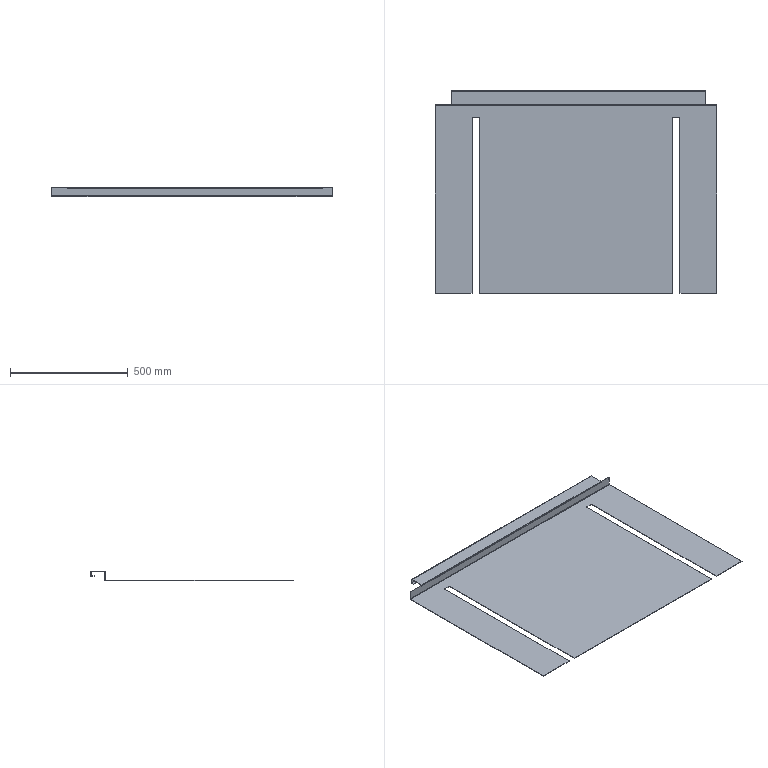Part | SolidWorks | features BaseBody 1 | 1 solid | 54 faces | box 1196 x 863 x 39 mm | volume 2108155 mm3 | plane 46 | cylinder 8 | commonest cylinder face diameters 2 x4 6 x4
STEP:
#1=CARTESIAN_POINT('',(412.5,349.,-2.));
#2=VERTEX_POINT('',#1);
#3=CARTESIAN_POINT('',(442.5,349.,-2.));
#4=VERTEX_POINT('',#3);
#5=CARTESIAN_POINT('',(412.5,349.,-2.));
#6=DIRECTION('',(1.,0.,0.));
#7=VECTOR('',#6,1000.);
#8=LINE('',#5,#7);
#9=EDGE_CURVE('',#2,#4,#8,.T.);
#10=ORIENTED_EDGE('',*,*,#9,.T.);
#11=CARTESIAN_POINT('',(442.5,349.,0.));
#12=VERTEX_POINT('',#11);
#13=CARTESIAN_POINT('',(442.5,349.,0.));
#14=DIRECTION('',(0.,0.,-1.));
#15=VECTOR('',#14,1000.);
#16=LINE('',#13,#15);
#17=EDGE_CURVE('',#12,#4,#16,.T.);
#18=ORIENTED_EDGE('',*,*,#17,.F.);
#19=CARTESIAN_POINT('',(412.5,349.,0.));
#20=VERTEX_POINT('',#19);
#21=CARTESIAN_POINT('',(412.5,349.,0.));
#22=DIRECTION('',(1.,0.,0.));
#23=VECTOR('',#22,1000.);
#24=LINE('',#21,#23);
#25=EDGE_CURVE('',#20,#12,#24,.T.);
#26=ORIENTED_EDGE('',*,*,#25,.F.);
#27=CARTESIAN_POINT('',(412.5,349.,0.));
#28=DIRECTION('',(0.,0.,-1.));
#29=VECTOR('',#28,1000.);
#30=LINE('',#27,#29);
#31=EDGE_CURVE('',#20,#2,#30,.T.);
#32=ORIENTED_EDGE('',*,*,#31,.T.);
#33=EDGE_LOOP('',(#10,#18,#26,#32));
#34=FACE_OUTER_BOUND('',#33,.T.);
#35=CARTESIAN_POINT('',(412.5,349.,0.));
#36=DIRECTION('',(0.,1.,0.));
#37=DIRECTION('',(1.,0.,0.));
#38=AXIS2_PLACEMENT_3D('',#35,#36,#37);
#39=PLANE('',#38);
#40=ADVANCED_FACE('',(#34),#39,.F.);
#41=CARTESIAN_POINT('',(442.5,-401.,-2.));
#42=VERTEX_POINT('',#41);
#43=CARTESIAN_POINT('',(442.5,349.,-2.));
#44=DIRECTION('',(0.,-1.,0.));
#45=VECTOR('',#44,1000.);
#46=LINE('',#43,#45);
#47=EDGE_CURVE('',#4,#42,#46,.T.);
#48=ORIENTED_EDGE('',*,*,#47,.T.);
#49=CARTESIAN_POINT('',(442.5,-401.,0.));
#50=VERTEX_POINT('',#49);
#51=CARTESIAN_POINT('',(442.5,-401.,0.));
#52=DIRECTION('',(0.,0.,-1.));
#53=VECTOR('',#52,1000.);
#54=LINE('',#51,#53);
#55=EDGE_CURVE('',#50,#42,#54,.T.);
#56=ORIENTED_EDGE('',*,*,#55,.F.);
#57=CARTESIAN_POINT('',(442.5,349.,0.));
#58=DIRECTION('',(0.,-1.,0.));
#59=VECTOR('',#58,1000.);
#60=LINE('',#57,#59);
#61=EDGE_CURVE('',#12,#50,#60,.T.);
#62=ORIENTED_EDGE('',*,*,#61,.F.);
#63=ORIENTED_EDGE('',*,*,#17,.T.);
#64=EDGE_LOOP('',(#48,#56,#62,#63));
#65=FACE_OUTER_BOUND('',#64,.T.);
#66=CARTESIAN_POINT('',(442.5,349.,0.));
#67=DIRECTION('',(1.,0.,0.));
#68=DIRECTION('',(0.,-1.,0.));
#69=AXIS2_PLACEMENT_3D('',#66,#67,#68);
#70=PLANE('',#69);
#71=ADVANCED_FACE('',(#65),#70,.F.);
#72=CARTESIAN_POINT('',(412.5,-401.,-2.));
#73=VERTEX_POINT('',#72);
#74=CARTESIAN_POINT('',(412.5,349.,-2.));
#75=DIRECTION('',(0.,1.,0.));
#76=VECTOR('',#75,1000.);
#77=LINE('',#74,#76);
#78=EDGE_CURVE('',#73,#2,#77,.T.);
#79=ORIENTED_EDGE('',*,*,#78,.T.);
#80=ORIENTED_EDGE('',*,*,#31,.F.);
#81=CARTESIAN_POINT('',(412.5,-401.,0.));
#82=VERTEX_POINT('',#81);
#83=CARTESIAN_POINT('',(412.5,349.,0.));
#84=DIRECTION('',(0.,1.,0.));
#85=VECTOR('',#84,1000.);
#86=LINE('',#83,#85);
#87=EDGE_CURVE('',#82,#20,#86,.T.);
#88=ORIENTED_EDGE('',*,*,#87,.F.);
#89=CARTESIAN_POINT('',(412.5,-401.,0.));
#90=DIRECTION('',(0.,0.,-1.));
#91=VECTOR('',#90,1000.);
#92=LINE('',#89,#91);
#93=EDGE_CURVE('',#82,#73,#92,.T.);
#94=ORIENTED_EDGE('',*,*,#93,.T.);
#95=EDGE_LOOP('',(#79,#80,#88,#94));
#96=FACE_OUTER_BOUND('',#95,.T.);
#97=CARTESIAN_POINT('',(412.5,349.,0.));
#98=DIRECTION('',(-1.,0.,0.));
#99=DIRECTION('',(0.,0.,1.));
#100=AXIS2_PLACEMENT_3D('',#97,#98,#99);
#101=PLANE('',#100);
#102=ADVANCED_FACE('',(#96),#101,.F.);
#103=CARTESIAN_POINT('',(-442.5,349.,-2.));
#104=VERTEX_POINT('',#103);
#105=CARTESIAN_POINT('',(-412.5,349.,-2.));
#106=VERTEX_POINT('',#105);
#107=CARTESIAN_POINT('',(-412.5,349.,-2.));
#108=DIRECTION('',(1.,0.,0.));
#109=VECTOR('',#108,1000.);
#110=LINE('',#107,#109);
#111=EDGE_CURVE('',#104,#106,#110,.T.);
#112=ORIENTED_EDGE('',*,*,#111,.T.);
#113=CARTESIAN_POINT('',(-412.5,349.,0.));
#114=VERTEX_POINT('',#113);
#115=CARTESIAN_POINT('',(-412.5,349.,0.));
#116=DIRECTION('',(0.,0.,-1.));
#117=VECTOR('',#116,1000.);
#118=LINE('',#115,#117);
#119=EDGE_CURVE('',#114,#106,#118,.T.);
#120=ORIENTED_EDGE('',*,*,#119,.F.);
#121=CARTESIAN_POINT('',(-442.5,349.,0.));
#122=VERTEX_POINT('',#121);
#123=CARTESIAN_POINT('',(-412.5,349.,0.));
#124=DIRECTION('',(1.,0.,0.));
#125=VECTOR('',#124,1000.);
#126=LINE('',#123,#125);
#127=EDGE_CURVE('',#122,#114,#126,.T.);
#128=ORIENTED_EDGE('',*,*,#127,.F.);
#129=CARTESIAN_POINT('',(-442.5,349.,0.));
#130=DIRECTION('',(0.,0.,-1.));
#131=VECTOR('',#130,1000.);
#132=LINE('',#129,#131);
#133=EDGE_CURVE('',#122,#104,#132,.T.);
#134=ORIENTED_EDGE('',*,*,#133,.T.);
#135=EDGE_LOOP('',(#112,#120,#128,#134));
#136=FACE_OUTER_BOUND('',#135,.T.);
#137=CARTESIAN_POINT('',(-412.5,349.,0.));
#138=DIRECTION('',(0.,1.,0.));
#139=DIRECTION('',(1.,0.,0.));
#140=AXIS2_PLACEMENT_3D('',#137,#138,#139);
#141=PLANE('',#140);
#142=ADVANCED_FACE('',(#136),#141,.F.);
#143=CARTESIAN_POINT('',(-412.5,-401.,-2.));
#144=VERTEX_POINT('',#143);
#145=CARTESIAN_POINT('',(-412.5,349.,-2.));
#146=DIRECTION('',(0.,-1.,0.));
#147=VECTOR('',#146,1000.);
#148=LINE('',#145,#147);
#149=EDGE_CURVE('',#106,#144,#148,.T.);
#150=ORIENTED_EDGE('',*,*,#149,.T.);
#151=CARTESIAN_POINT('',(-412.5,-401.,0.));
#152=VERTEX_POINT('',#151);
#153=CARTESIAN_POINT('',(-412.5,-401.,0.));
#154=DIRECTION('',(0.,0.,-1.));
#155=VECTOR('',#154,1000.);
#156=LINE('',#153,#155);
#157=EDGE_CURVE('',#152,#144,#156,.T.);
#158=ORIENTED_EDGE('',*,*,#157,.F.);
#159=CARTESIAN_POINT('',(-412.5,349.,0.));
#160=DIRECTION('',(0.,-1.,0.));
#161=VECTOR('',#160,1000.);
#162=LINE('',#159,#161);
#163=EDGE_CURVE('',#114,#152,#162,.T.);
#164=ORIENTED_EDGE('',*,*,#163,.F.);
#165=ORIENTED_EDGE('',*,*,#119,.T.);
#166=EDGE_LOOP('',(#150,#158,#164,#165));
#167=FACE_OUTER_BOUND('',#166,.T.);
#168=CARTESIAN_POINT('',(-412.5,349.,0.));
#169=DIRECTION('',(1.,0.,0.));
#170=DIRECTION('',(0.,-1.,0.));
#171=AXIS2_PLACEMENT_3D('',#168,#169,#170);
#172=PLANE('',#171);
#173=ADVANCED_FACE('',(#167),#172,.F.);
#174=CARTESIAN_POINT('',(-442.5,-401.,-2.));
#175=VERTEX_POINT('',#174);
#176=CARTESIAN_POINT('',(-442.5,349.,-2.));
#177=DIRECTION('',(0.,1.,0.));
#178=VECTOR('',#177,1000.);
#179=LINE('',#176,#178);
#180=EDGE_CURVE('',#175,#104,#179,.T.);
#181=ORIENTED_EDGE('',*,*,#180,.T.);
#182=ORIENTED_EDGE('',*,*,#133,.F.);
#183=CARTESIAN_POINT('',(-442.5,-401.,0.));
#184=VERTEX_POINT('',#183);
#185=CARTESIAN_POINT('',(-442.5,349.,0.));
#186=DIRECTION('',(0.,1.,0.));
#187=VECTOR('',#186,1000.);
#188=LINE('',#185,#187);
#189=EDGE_CURVE('',#184,#122,#188,.T.);
#190=ORIENTED_EDGE('',*,*,#189,.F.);
#191=CARTESIAN_POINT('',(-442.5,-401.,0.));
#192=DIRECTION('',(0.,0.,-1.));
#193=VECTOR('',#192,1000.);
#194=LINE('',#191,#193);
#195=EDGE_CURVE('',#184,#175,#194,.T.);
#196=ORIENTED_EDGE('',*,*,#195,.T.);
#197=EDGE_LOOP('',(#181,#182,#190,#196));
#198=FACE_OUTER_BOUND('',#197,.T.);
#199=CARTESIAN_POINT('',(-442.5,349.,0.));
#200=DIRECTION('',(-1.,0.,0.));
#201=DIRECTION('',(0.,0.,1.));
#202=AXIS2_PLACEMENT_3D('',#199,#200,#201);
#203=PLANE('',#202);
#204=ADVANCED_FACE('',(#198),#203,.F.);
#205=CARTESIAN_POINT('',(-528.,447.,19.));
#206=VERTEX_POINT('',#205);
#207=CARTESIAN_POINT('',(553.,447.,19.));
#208=VERTEX_POINT('',#207);
#209=CARTESIAN_POINT('',(0.,447.,19.));
#210=DIRECTION('',(1.,0.,0.));
#211=VECTOR('',#210,1000.);
#212=LINE('',#209,#211);
#213=EDGE_CURVE('',#206,#208,#212,.T.);
#214=ORIENTED_EDGE('',*,*,#213,.F.);
#215=CARTESIAN_POINT('',(-528.,447.,17.));
#216=VERTEX_POINT('',#215);
#217=CARTESIAN_POINT('',(-528.,447.,17.));
#218=DIRECTION('',(0.,0.,1.));
#219=VECTOR('',#218,1000.);
#220=LINE('',#217,#219);
#221=EDGE_CURVE('',#216,#206,#220,.T.);
#222=ORIENTED_EDGE('',*,*,#221,.F.);
#223=CARTESIAN_POINT('',(553.,447.,17.));
#224=VERTEX_POINT('',#223);
#225=CARTESIAN_POINT('',(553.,447.,17.));
#226=DIRECTION('',(1.,0.,0.));
#227=VECTOR('',#226,1000.);
#228=LINE('',#225,#227);
#229=EDGE_CURVE('',#216,#224,#228,.T.);
#230=ORIENTED_EDGE('',*,*,#229,.T.);
#231=CARTESIAN_POINT('',(553.,447.,17.));
#232=DIRECTION('',(0.,0.,1.));
#233=VECTOR('',#232,1000.);
#234=LINE('',#231,#233);
#235=EDGE_CURVE('',#224,#208,#234,.T.);
#236=ORIENTED_EDGE('',*,*,#235,.T.);
#237=EDGE_LOOP('',(#214,#222,#230,#236));
#238=FACE_OUTER_BOUND('',#237,.T.);
#239=CARTESIAN_POINT('',(553.,447.,17.));
#240=DIRECTION('',(0.,-1.,0.));
#241=DIRECTION('',(0.,0.,-1.));
#242=AXIS2_PLACEMENT_3D('',#239,#240,#241);
#243=PLANE('',#242);
#244=ADVANCED_FACE('',(#238),#243,.T.);
#245=CARTESIAN_POINT('',(-528.,459.,19.));
#246=VERTEX_POINT('',#245);
#247=CARTESIAN_POINT('',(553.,459.,19.));
#248=VERTEX_POINT('',#247);
#249=CARTESIAN_POINT('',(-528.,459.,19.));
#250=DIRECTION('',(1.,0.,0.));
#251=VECTOR('',#250,1000.);
#252=LINE('',#249,#251);
#253=EDGE_CURVE('',#246,#248,#252,.T.);
#254=ORIENTED_EDGE('',*,*,#253,.F.);
#255=CARTESIAN_POINT('',(-528.,0.,19.));
#256=DIRECTION('',(0.,-1.,0.));
#257=VECTOR('',#256,1000.);
#258=LINE('',#255,#257);
#259=EDGE_CURVE('',#246,#206,#258,.T.);
#260=ORIENTED_EDGE('',*,*,#259,.T.);
#261=ORIENTED_EDGE('',*,*,#213,.T.);
#262=CARTESIAN_POINT('',(553.,0.,19.));
#263=DIRECTION('',(0.,1.,0.));
#264=VECTOR('',#263,1000.);
#265=LINE('',#262,#264);
#266=EDGE_CURVE('',#208,#248,#265,.T.);
#267=ORIENTED_EDGE('',*,*,#266,.T.);
#268=EDGE_LOOP('',(#254,#260,#261,#267));
#269=FACE_OUTER_BOUND('',#268,.T.);
#270=CARTESIAN_POINT('',(0.,0.,19.));
#271=DIRECTION('',(0.,0.,-1.));
#272=DIRECTION('',(-1.,0.,0.));
#273=AXIS2_PLACEMENT_3D('',#270,#271,#272);
#274=PLANE('',#273);
#275=ADVANCED_FACE('',(#269),#274,.F.);
#276=CARTESIAN_POINT('',(-528.,459.,17.));
#277=VERTEX_POINT('',#276);
#278=CARTESIAN_POINT('',(-528.,447.,17.));
#279=DIRECTION('',(0.,-1.,0.));
#280=VECTOR('',#279,1000.);
#281=LINE('',#278,#280);
#282=EDGE_CURVE('',#277,#216,#281,.T.);
#283=ORIENTED_EDGE('',*,*,#282,.F.);
#284=CARTESIAN_POINT('',(553.,459.,17.));
#285=VERTEX_POINT('',#284);
#286=CARTESIAN_POINT('',(0.,459.,17.));
#287=DIRECTION('',(1.,0.,0.));
#288=VECTOR('',#287,1000.);
#289=LINE('',#286,#288);
#290=EDGE_CURVE('',#277,#285,#289,.T.);
#291=ORIENTED_EDGE('',*,*,#290,.T.);
#292=CARTESIAN_POINT('',(553.,460.,17.));
#293=DIRECTION('',(0.,1.,0.));
#294=VECTOR('',#293,1000.);
#295=LINE('',#292,#294);
#296=EDGE_CURVE('',#224,#285,#295,.T.);
#297=ORIENTED_EDGE('',*,*,#296,.F.);
#298=ORIENTED_EDGE('',*,*,#229,.F.);
#299=EDGE_LOOP('',(#283,#291,#297,#298));
#300=FACE_OUTER_BOUND('',#299,.T.);
#301=CARTESIAN_POINT('',(0.,0.,17.));
#302=DIRECTION('',(0.,0.,-1.));
#303=DIRECTION('',(-1.,0.,0.));
#304=AXIS2_PLACEMENT_3D('',#301,#302,#303);
#305=PLANE('',#304);
#306=ADVANCED_FACE('',(#300),#305,.T.);
#307=ORIENTED_EDGE('',*,*,#259,.F.);
#308=CARTESIAN_POINT('',(-528.,459.,17.));
#309=DIRECTION('',(0.,0.,-1.));
#310=VECTOR('',#309,1000.);
#311=LINE('',#308,#310);
#312=EDGE_CURVE('',#246,#277,#311,.T.);
#313=ORIENTED_EDGE('',*,*,#312,.T.);
#314=ORIENTED_EDGE('',*,*,#282,.T.);
#315=ORIENTED_EDGE('',*,*,#221,.T.);
#316=EDGE_LOOP('',(#307,#313,#314,#315));
#317=FACE_OUTER_BOUND('',#316,.T.);
#318=CARTESIAN_POINT('',(-528.,447.,17.));
#319=DIRECTION('',(-1.,0.,0.));
#320=DIRECTION('',(0.,0.,1.));
#321=AXIS2_PLACEMENT_3D('',#318,#319,#320);
#322=PLANE('',#321);
#323=ADVANCED_FACE('',(#317),#322,.T.);
#324=ORIENTED_EDGE('',*,*,#296,.T.);
#325=CARTESIAN_POINT('',(553.,459.,19.));
#326=DIRECTION('',(0.,0.,-1.));
#327=VECTOR('',#326,1000.);
#328=LINE('',#325,#327);
#329=EDGE_CURVE('',#248,#285,#328,.T.);
#330=ORIENTED_EDGE('',*,*,#329,.F.);
#331=ORIENTED_EDGE('',*,*,#266,.F.);
#332=ORIENTED_EDGE('',*,*,#235,.F.);
#333=EDGE_LOOP('',(#324,#330,#331,#332));
#334=FACE_OUTER_BOUND('',#333,.T.);
#335=CARTESIAN_POINT('',(553.,460.,17.));
#336=DIRECTION('',(1.,0.,0.));
#337=DIRECTION('',(0.,1.,0.));
#338=AXIS2_PLACEMENT_3D('',#335,#336,#337);
#339=PLANE('',#338);
#340=ADVANCED_FACE('',(#334),#339,.T.);
#341=CARTESIAN_POINT('',(553.,460.,20.));
#342=VERTEX_POINT('',#341);
#343=CARTESIAN_POINT('',(-528.,460.,20.));
#344=VERTEX_POINT('',#343);
#345=CARTESIAN_POINT('',(553.,460.,20.));
#346=DIRECTION('',(-1.,0.,0.));
#347=VECTOR('',#346,1000.);
#348=LINE('',#345,#347);
#349=EDGE_CURVE('',#342,#344,#348,.T.);
#350=ORIENTED_EDGE('',*,*,#349,.T.);
#351=CARTESIAN_POINT('',(-528.,459.,20.));
#352=DIRECTION('',(-1.,0.,0.));
#353=DIRECTION('',(0.,0.,-1.));
#354=AXIS2_PLACEMENT_3D('',#351,#352,#353);
#355=CIRCLE('',#354,1.);
#356=EDGE_CURVE('',#344,#246,#355,.T.);
#357=ORIENTED_EDGE('',*,*,#356,.T.);
#358=ORIENTED_EDGE('',*,*,#253,.T.);
#359=CARTESIAN_POINT('',(553.,459.,20.));
#360=DIRECTION('',(1.,0.,0.));
#361=DIRECTION('',(0.,0.,-1.));
#362=AXIS2_PLACEMENT_3D('',#359,#360,#361);
#363=CIRCLE('',#362,1.);
#364=EDGE_CURVE('',#248,#342,#363,.T.);
#365=ORIENTED_EDGE('',*,*,#364,.T.);
#366=EDGE_LOOP('',(#350,#357,#358,#365));
#367=FACE_OUTER_BOUND('',#366,.T.);
#368=CARTESIAN_POINT('',(553.,459.,20.));
#369=DIRECTION('',(1.,0.,0.));
#370=DIRECTION('',(0.,0.,-1.));
#371=AXIS2_PLACEMENT_3D('',#368,#369,#370);
#372=CYLINDRICAL_SURFACE('',#371,1.);
#373=ADVANCED_FACE('',(#367),#372,.F.);
#374=CARTESIAN_POINT('',(553.,462.,20.));
#375=VERTEX_POINT('',#374);
#376=CARTESIAN_POINT('',(-528.,462.,20.));
#377=VERTEX_POINT('',#376);
#378=CARTESIAN_POINT('',(553.,462.,20.));
#379=DIRECTION('',(-1.,0.,0.));
#380=VECTOR('',#379,1000.);
#381=LINE('',#378,#380);
#382=EDGE_CURVE('',#375,#377,#381,.T.);
#383=ORIENTED_EDGE('',*,*,#382,.F.);
#384=CARTESIAN_POINT('',(553.,459.,20.));
#385=DIRECTION('',(1.,0.,0.));
#386=DIRECTION('',(0.,0.,-1.));
#387=AXIS2_PLACEMENT_3D('',#384,#385,#386);
#388=CIRCLE('',#387,3.);
#389=EDGE_CURVE('',#285,#375,#388,.T.);
#390=ORIENTED_EDGE('',*,*,#389,.F.);
#391=ORIENTED_EDGE('',*,*,#290,.F.);
#392=CARTESIAN_POINT('',(-528.,459.,20.));
#393=DIRECTION('',(-1.,0.,0.));
#394=DIRECTION('',(0.,0.,-1.));
#395=AXIS2_PLACEMENT_3D('',#392,#393,#394);
#396=CIRCLE('',#395,3.);
#397=EDGE_CURVE('',#377,#277,#396,.T.);
#398=ORIENTED_EDGE('',*,*,#397,.F.);
#399=EDGE_LOOP('',(#383,#390,#391,#398));
#400=FACE_OUTER_BOUND('',#399,.T.);
#401=CARTESIAN_POINT('',(553.,459.,20.));
#402=DIRECTION('',(1.,0.,0.));
#403=DIRECTION('',(0.,0.,-1.));
#404=AXIS2_PLACEMENT_3D('',#401,#402,#403);
#405=CYLINDRICAL_SURFACE('',#404,3.);
#406=ADVANCED_FACE('',(#400),#405,.T.);
#407=ORIENTED_EDGE('',*,*,#364,.F.);
#408=ORIENTED_EDGE('',*,*,#329,.T.);
#409=ORIENTED_EDGE('',*,*,#389,.T.);
#410=CARTESIAN_POINT('',(553.,460.,20.));
#411=DIRECTION('',(0.,1.,0.));
#412=VECTOR('',#411,1000.);
#413=LINE('',#410,#412);
#414=EDGE_CURVE('',#342,#375,#413,.T.);
#415=ORIENTED_EDGE('',*,*,#414,.F.);
#416=EDGE_LOOP('',(#407,#408,#409,#415));
#417=FACE_OUTER_BOUND('',#416,.T.);
#418=CARTESIAN_POINT('',(553.,459.,20.));
#419=DIRECTION('',(-1.,0.,0.));
#420=DIRECTION('',(0.,0.,1.));
#421=AXIS2_PLACEMENT_3D('',#418,#419,#420);
#422=PLANE('',#421);
#423=ADVANCED_FACE('',(#417),#422,.F.);
#424=ORIENTED_EDGE('',*,*,#312,.F.);
#425=ORIENTED_EDGE('',*,*,#356,.F.);
#426=CARTESIAN_POINT('',(-528.,460.,20.));
#427=DIRECTION('',(0.,1.,0.));
#428=VECTOR('',#427,1000.);
#429=LINE('',#426,#428);
#430=EDGE_CURVE('',#344,#377,#429,.T.);
#431=ORIENTED_EDGE('',*,*,#430,.T.);
#432=ORIENTED_EDGE('',*,*,#397,.T.);
#433=EDGE_LOOP('',(#424,#425,#431,#432));
#434=FACE_OUTER_BOUND('',#433,.T.);
#435=CARTESIAN_POINT('',(-528.,459.,20.));
#436=DIRECTION('',(-1.,0.,0.));
#437=DIRECTION('',(0.,0.,1.));
#438=AXIS2_PLACEMENT_3D('',#435,#436,#437);
#439=PLANE('',#438);
#440=ADVANCED_FACE('',(#434),#439,.T.);
#441=CARTESIAN_POINT('',(553.,459.,35.));
#442=VERTEX_POINT('',#441);
#443=CARTESIAN_POINT('',(-528.,459.,35.));
#444=VERTEX_POINT('',#443);
#445=CARTESIAN_POINT('',(553.,459.,35.));
#446=DIRECTION('',(-1.,0.,0.));
#447=VECTOR('',#446,1000.);
#448=LINE('',#445,#447);
#449=EDGE_CURVE('',#442,#444,#448,.T.);
#450=ORIENTED_EDGE('',*,*,#449,.T.);
#451=CARTESIAN_POINT('',(-528.,460.,34.));
#452=VERTEX_POINT('',#451);
#453=CARTESIAN_POINT('',(-528.,459.,34.));
#454=DIRECTION('',(-1.,0.,0.));
#455=DIRECTION('',(0.,0.,-1.));
#456=AXIS2_PLACEMENT_3D('',#453,#454,#455);
#457=CIRCLE('',#456,1.);
#458=EDGE_CURVE('',#444,#452,#457,.T.);
#459=ORIENTED_EDGE('',*,*,#458,.T.);
#460=CARTESIAN_POINT('',(553.,460.,34.));
#461=VERTEX_POINT('',#460);
#462=CARTESIAN_POINT('',(-528.,460.,34.));
#463=DIRECTION('',(1.,0.,0.));
#464=VECTOR('',#463,1000.);
#465=LINE('',#462,#464);
#466=EDGE_CURVE('',#452,#461,#465,.T.);
#467=ORIENTED_EDGE('',*,*,#466,.T.);
#468=CARTESIAN_POINT('',(553.,459.,34.));
#469=DIRECTION('',(1.,0.,0.));
#470=DIRECTION('',(0.,0.,-1.));
#471=AXIS2_PLACEMENT_3D('',#468,#469,#470);
#472=CIRCLE('',#471,1.);
#473=EDGE_CURVE('',#461,#442,#472,.T.);
#474=ORIENTED_EDGE('',*,*,#473,.T.);
#475=EDGE_LOOP('',(#450,#459,#467,#474));
#476=FACE_OUTER_BOUND('',#475,.T.);
#477=CARTESIAN_POINT('',(553.,459.,34.));
#478=DIRECTION('',(1.,0.,0.));
#479=DIRECTION('',(0.,1.,0.));
#480=AXIS2_PLACEMENT_3D('',#477,#478,#479);
#481=CYLINDRICAL_SURFACE('',#480,1.);
#482=ADVANCED_FACE('',(#476),#481,.F.);
#483=CARTESIAN_POINT('',(553.,459.,37.));
#484=VERTEX_POINT('',#483);
#485=CARTESIAN_POINT('',(-528.,459.,37.));
#486=VERTEX_POINT('',#485);
#487=CARTESIAN_POINT('',(553.,459.,37.));
#488=DIRECTION('',(-1.,0.,0.));
#489=VECTOR('',#488,1000.);
#490=LINE('',#487,#489);
#491=EDGE_CURVE('',#484,#486,#490,.T.);
#492=ORIENTED_EDGE('',*,*,#491,.F.);
#493=CARTESIAN_POINT('',(553.,462.,34.));
#494=VERTEX_POINT('',#493);
#495=CARTESIAN_POINT('',(553.,459.,34.));
#496=DIRECTION('',(1.,0.,0.));
#497=DIRECTION('',(0.,0.,-1.));
#498=AXIS2_PLACEMENT_3D('',#495,#496,#497);
#499=CIRCLE('',#498,3.);
#500=EDGE_CURVE('',#494,#484,#499,.T.);
#501=ORIENTED_EDGE('',*,*,#500,.F.);
#502=CARTESIAN_POINT('',(-528.,462.,34.));
#503=VERTEX_POINT('',#502);
#504=CARTESIAN_POINT('',(-528.,462.,34.));
#505=DIRECTION('',(-1.,0.,0.));
#506=VECTOR('',#505,1000.);
#507=LINE('',#504,#506);
#508=EDGE_CURVE('',#494,#503,#507,.T.);
#509=ORIENTED_EDGE('',*,*,#508,.T.);
#510=CARTESIAN_POINT('',(-528.,459.,34.));
#511=DIRECTION('',(-1.,0.,0.));
#512=DIRECTION('',(0.,0.,-1.));
#513=AXIS2_PLACEMENT_3D('',#510,#511,#512);
#514=CIRCLE('',#513,3.);
#515=EDGE_CURVE('',#486,#503,#514,.T.);
#516=ORIENTED_EDGE('',*,*,#515,.F.);
#517=EDGE_LOOP('',(#492,#501,#509,#516));
#518=FACE_OUTER_BOUND('',#517,.T.);
#519=CARTESIAN_POINT('',(553.,459.,34.));
#520=DIRECTION('',(1.,0.,0.));
#521=DIRECTION('',(0.,1.,0.));
#522=AXIS2_PLACEMENT_3D('',#519,#520,#521);
#523=CYLINDRICAL_SURFACE('',#522,3.);
#524=ADVANCED_FACE('',(#518),#523,.T.);
#525=ORIENTED_EDGE('',*,*,#473,.F.);
#526=CARTESIAN_POINT('',(553.,460.,34.));
#527=DIRECTION('',(0.,1.,0.));
#528=VECTOR('',#527,1000.);
#529=LINE('',#526,#528);
#530=EDGE_CURVE('',#461,#494,#529,.T.);
#531=ORIENTED_EDGE('',*,*,#530,.T.);
#532=ORIENTED_EDGE('',*,*,#500,.T.);
#533=CARTESIAN_POINT('',(553.,459.,35.));
#534=DIRECTION('',(0.,0.,1.));
#535=VECTOR('',#534,1000.);
#536=LINE('',#533,#535);
#537=EDGE_CURVE('',#442,#484,#536,.T.);
#538=ORIENTED_EDGE('',*,*,#537,.F.);
#539=EDGE_LOOP('',(#525,#531,#532,#538));
#540=FACE_OUTER_BOUND('',#539,.T.);
#541=CARTESIAN_POINT('',(553.,459.,34.));
#542=DIRECTION('',(-1.,0.,0.));
#543=DIRECTION('',(0.,0.,1.));
#544=AXIS2_PLACEMENT_3D('',#541,#542,#543);
#545=PLANE('',#544);
#546=ADVANCED_FACE('',(#540),#545,.F.);
#547=CARTESIAN_POINT('',(-528.,462.,34.));
#548=DIRECTION('',(0.,1.,0.));
#549=VECTOR('',#548,1000.);
#550=LINE('',#547,#549);
#551=EDGE_CURVE('',#452,#503,#550,.T.);
#552=ORIENTED_EDGE('',*,*,#551,.F.);
#553=ORIENTED_EDGE('',*,*,#458,.F.);
#554=CARTESIAN_POINT('',(-528.,459.,35.));
#555=DIRECTION('',(0.,0.,1.));
#556=VECTOR('',#555,1000.);
#557=LINE('',#554,#556);
#558=EDGE_CURVE('',#444,#486,#557,.T.);
#559=ORIENTED_EDGE('',*,*,#558,.T.);
#560=ORIENTED_EDGE('',*,*,#515,.T.);
#561=EDGE_LOOP('',(#552,#553,#559,#560));
#562=FACE_OUTER_BOUND('',#561,.T.);
#563=CARTESIAN_POINT('',(-528.,459.,34.));
#564=DIRECTION('',(-1.,0.,0.));
#565=DIRECTION('',(0.,0.,1.));
#566=AXIS2_PLACEMENT_3D('',#563,#564,#565);
#567=PLANE('',#566);
#568=ADVANCED_FACE('',(#562),#567,.T.);
#569=CARTESIAN_POINT('',(553.,401.,34.));
#570=VERTEX_POINT('',#569);
#571=CARTESIAN_POINT('',(-528.,401.,34.));
#572=VERTEX_POINT('',#571);
#573=CARTESIAN_POINT('',(553.,401.,34.));
#574=DIRECTION('',(-1.,0.,0.));
#575=VECTOR('',#574,1000.);
#576=LINE('',#573,#575);
#577=EDGE_CURVE('',#570,#572,#576,.T.);
#578=ORIENTED_EDGE('',*,*,#577,.T.);
#579=CARTESIAN_POINT('',(-528.,402.,35.));
#580=VERTEX_POINT('',#579);
#581=CARTESIAN_POINT('',(-528.,402.,34.));
#582=DIRECTION('',(-1.,0.,0.));
#583=DIRECTION('',(0.,0.,-1.));
#584=AXIS2_PLACEMENT_3D('',#581,#582,#583);
#585=CIRCLE('',#584,1.);
#586=EDGE_CURVE('',#572,#580,#585,.T.);
#587=ORIENTED_EDGE('',*,*,#586,.T.);
#588=CARTESIAN_POINT('',(553.,402.,35.));
#589=VERTEX_POINT('',#588);
#590=CARTESIAN_POINT('',(-528.,402.,35.));
#591=DIRECTION('',(1.,0.,0.));
#592=VECTOR('',#591,1000.);
#593=LINE('',#590,#592);
#594=EDGE_CURVE('',#580,#589,#593,.T.);
#595=ORIENTED_EDGE('',*,*,#594,.T.);
#596=CARTESIAN_POINT('',(553.,402.,34.));
#597=DIRECTION('',(1.,0.,0.));
#598=DIRECTION('',(0.,0.,-1.));
#599=AXIS2_PLACEMENT_3D('',#596,#597,#598);
#600=CIRCLE('',#599,1.);
#601=EDGE_CURVE('',#589,#570,#600,.T.);
#602=ORIENTED_EDGE('',*,*,#601,.T.);
#603=EDGE_LOOP('',(#578,#587,#595,#602));
#604=FACE_OUTER_BOUND('',#603,.T.);
#605=CARTESIAN_POINT('',(553.,402.,34.));
#606=DIRECTION('',(1.,0.,0.));
#607=DIRECTION('',(0.,0.,1.));
#608=AXIS2_PLACEMENT_3D('',#605,#606,#607);
#609=CYLINDRICAL_SURFACE('',#608,1.);
#610=ADVANCED_FACE('',(#604),#609,.F.);
#611=CARTESIAN_POINT('',(553.,399.,34.));
#612=VERTEX_POINT('',#611);
#613=CARTESIAN_POINT('',(-528.,399.,34.));
#614=VERTEX_POINT('',#613);
#615=CARTESIAN_POINT('',(553.,399.,34.));
#616=DIRECTION('',(-1.,0.,0.));
#617=VECTOR('',#616,1000.);
#618=LINE('',#615,#617);
#619=EDGE_CURVE('',#612,#614,#618,.T.);
#620=ORIENTED_EDGE('',*,*,#619,.F.);
#621=CARTESIAN_POINT('',(553.,402.,37.));
#622=VERTEX_POINT('',#621);
#623=CARTESIAN_POINT('',(553.,402.,34.));
#624=DIRECTION('',(1.,0.,0.));
#625=DIRECTION('',(0.,0.,-1.));
#626=AXIS2_PLACEMENT_3D('',#623,#624,#625);
#627=CIRCLE('',#626,3.);
#628=EDGE_CURVE('',#622,#612,#627,.T.);
#629=ORIENTED_EDGE('',*,*,#628,.F.);
#630=CARTESIAN_POINT('',(-528.,402.,37.));
#631=VERTEX_POINT('',#630);
#632=CARTESIAN_POINT('',(-528.,402.,37.));
#633=DIRECTION('',(-1.,0.,0.));
#634=VECTOR('',#633,1000.);
#635=LINE('',#632,#634);
#636=EDGE_CURVE('',#622,#631,#635,.T.);
#637=ORIENTED_EDGE('',*,*,#636,.T.);
#638=CARTESIAN_POINT('',(-528.,402.,34.));
#639=DIRECTION('',(-1.,0.,0.));
#640=DIRECTION('',(0.,0.,-1.));
#641=AXIS2_PLACEMENT_3D('',#638,#639,#640);
#642=CIRCLE('',#641,3.);
#643=EDGE_CURVE('',#614,#631,#642,.T.);
#644=ORIENTED_EDGE('',*,*,#643,.F.);
#645=EDGE_LOOP('',(#620,#629,#637,#644));
#646=FACE_OUTER_BOUND('',#645,.T.);
#647=CARTESIAN_POINT('',(553.,402.,34.));
#648=DIRECTION('',(1.,0.,0.));
#649=DIRECTION('',(0.,0.,1.));
#650=AXIS2_PLACEMENT_3D('',#647,#648,#649);
#651=CYLINDRICAL_SURFACE('',#650,3.);
#652=ADVANCED_FACE('',(#646),#651,.T.);
#653=ORIENTED_EDGE('',*,*,#601,.F.);
#654=CARTESIAN_POINT('',(553.,402.,35.));
#655=DIRECTION('',(0.,0.,1.));
#656=VECTOR('',#655,1000.);
#657=LINE('',#654,#656);
#658=EDGE_CURVE('',#589,#622,#657,.T.);
#659=ORIENTED_EDGE('',*,*,#658,.T.);
#660=ORIENTED_EDGE('',*,*,#628,.T.);
#661=CARTESIAN_POINT('',(553.,401.,34.));
#662=DIRECTION('',(0.,-1.,0.));
#663=VECTOR('',#662,1000.);
#664=LINE('',#661,#663);
#665=EDGE_CURVE('',#570,#612,#664,.T.);
#666=ORIENTED_EDGE('',*,*,#665,.F.);
#667=EDGE_LOOP('',(#653,#659,#660,#666));
#668=FACE_OUTER_BOUND('',#667,.T.);
#669=CARTESIAN_POINT('',(553.,402.,34.));
#670=DIRECTION('',(-1.,0.,0.));
#671=DIRECTION('',(0.,0.,1.));
#672=AXIS2_PLACEMENT_3D('',#669,#670,#671);
#673=PLANE('',#672);
#674=ADVANCED_FACE('',(#668),#673,.F.);
#675=CARTESIAN_POINT('',(-528.,402.,37.));
#676=DIRECTION('',(0.,0.,1.));
#677=VECTOR('',#676,1000.);
#678=LINE('',#675,#677);
#679=EDGE_CURVE('',#580,#631,#678,.T.);
#680=ORIENTED_EDGE('',*,*,#679,.F.);
#681=ORIENTED_EDGE('',*,*,#586,.F.);
#682=CARTESIAN_POINT('',(-528.,401.,34.));
#683=DIRECTION('',(0.,-1.,0.));
#684=VECTOR('',#683,1000.);
#685=LINE('',#682,#684);
#686=EDGE_CURVE('',#572,#614,#685,.T.);
#687=ORIENTED_EDGE('',*,*,#686,.T.);
#688=ORIENTED_EDGE('',*,*,#643,.T.);
#689=EDGE_LOOP('',(#680,#681,#687,#688));
#690=FACE_OUTER_BOUND('',#689,.T.);
#691=CARTESIAN_POINT('',(-528.,402.,34.));
#692=DIRECTION('',(-1.,0.,0.));
#693=DIRECTION('',(0.,0.,1.));
#694=AXIS2_PLACEMENT_3D('',#691,#692,#693);
#695=PLANE('',#694);
#696=ADVANCED_FACE('',(#690),#695,.T.);
#697=CARTESIAN_POINT('',(-529.,399.,33.));
#698=VERTEX_POINT('',#697);
#699=CARTESIAN_POINT('',(-529.,399.,37.));
#700=VERTEX_POINT('',#699);
#701=CARTESIAN_POINT('',(-529.,399.,0.));
#702=DIRECTION('',(0.,0.,1.));
#703=VECTOR('',#702,1000.);
#704=LINE('',#701,#703);
#705=EDGE_CURVE('',#698,#700,#704,.T.);
#706=ORIENTED_EDGE('',*,*,#705,.F.);
#707=CARTESIAN_POINT('',(-529.,401.,33.));
#708=VERTEX_POINT('',#707);
#709=CARTESIAN_POINT('',(-529.,401.,33.));
#710=DIRECTION('',(0.,-1.,0.));
#711=VECTOR('',#710,1000.);
#712=LINE('',#709,#711);
#713=EDGE_CURVE('',#708,#698,#712,.T.);
#714=ORIENTED_EDGE('',*,*,#713,.F.);
#715=CARTESIAN_POINT('',(-529.,401.,37.));
#716=VERTEX_POINT('',#715);
#717=CARTESIAN_POINT('',(-529.,401.,33.));
#718=DIRECTION('',(0.,0.,1.));
#719=VECTOR('',#718,1000.);
#720=LINE('',#717,#719);
#721=EDGE_CURVE('',#708,#716,#720,.T.);
#722=ORIENTED_EDGE('',*,*,#721,.T.);
#723=CARTESIAN_POINT('',(-529.,401.,37.));
#724=DIRECTION('',(0.,-1.,0.));
#725=VECTOR('',#724,1000.);
#726=LINE('',#723,#725);
#727=EDGE_CURVE('',#716,#700,#726,.T.);
#728=ORIENTED_EDGE('',*,*,#727,.T.);
#729=EDGE_LOOP('',(#706,#714,#722,#728));
#730=FACE_OUTER_BOUND('',#729,.T.);
#731=CARTESIAN_POINT('',(-529.,401.,33.));
#732=DIRECTION('',(1.,0.,0.));
#733=DIRECTION('',(0.,1.,0.));
#734=AXIS2_PLACEMENT_3D('',#731,#732,#733);
#735=PLANE('',#734);
#736=ADVANCED_FACE('',(#730),#735,.T.);
#737=CARTESIAN_POINT('',(-528.,399.,33.));
#738=VERTEX_POINT('',#737);
#739=CARTESIAN_POINT('',(0.,399.,33.));
#740=DIRECTION('',(-1.,0.,0.));
#741=VECTOR('',#740,1000.);
#742=LINE('',#739,#741);
#743=EDGE_CURVE('',#738,#698,#742,.T.);
#744=ORIENTED_EDGE('',*,*,#743,.F.);
#745=CARTESIAN_POINT('',(-528.,401.,33.));
#746=VERTEX_POINT('',#745);
#747=CARTESIAN_POINT('',(-528.,401.,33.));
#748=DIRECTION('',(0.,-1.,0.));
#749=VECTOR('',#748,1000.);
#750=LINE('',#747,#749);
#751=EDGE_CURVE('',#746,#738,#750,.T.);
#752=ORIENTED_EDGE('',*,*,#751,.F.);
#753=CARTESIAN_POINT('',(-528.,401.,33.));
#754=DIRECTION('',(-1.,0.,0.));
#755=VECTOR('',#754,1000.);
#756=LINE('',#753,#755);
#757=EDGE_CURVE('',#746,#708,#756,.T.);
#758=ORIENTED_EDGE('',*,*,#757,.T.);
#759=ORIENTED_EDGE('',*,*,#713,.T.);
#760=EDGE_LOOP('',(#744,#752,#758,#759));
#761=FACE_OUTER_BOUND('',#760,.T.);
#762=CARTESIAN_POINT('',(-528.,401.,33.));
#763=DIRECTION('',(0.,0.,1.));
#764=DIRECTION('',(0.,-1.,0.));
#765=AXIS2_PLACEMENT_3D('',#762,#763,#764);
#766=PLANE('',#765);
#767=ADVANCED_FACE('',(#761),#766,.T.);
#768=CARTESIAN_POINT('',(-528.,399.,0.));
#769=DIRECTION('',(0.,0.,-1.));
#770=VECTOR('',#769,1000.);
#771=LINE('',#768,#770);
#772=EDGE_CURVE('',#614,#738,#771,.T.);
#773=ORIENTED_EDGE('',*,*,#772,.F.);
#774=ORIENTED_EDGE('',*,*,#686,.F.);
#775=CARTESIAN_POINT('',(-528.,401.,34.));
#776=DIRECTION('',(0.,0.,-1.));
#777=VECTOR('',#776,1000.);
#778=LINE('',#775,#777);
#779=EDGE_CURVE('',#572,#746,#778,.T.);
#780=ORIENTED_EDGE('',*,*,#779,.T.);
#781=ORIENTED_EDGE('',*,*,#751,.T.);
#782=EDGE_LOOP('',(#773,#774,#780,#781));
#783=FACE_OUTER_BOUND('',#782,.T.);
#784=CARTESIAN_POINT('',(-528.,401.,34.));
#785=DIRECTION('',(-1.,0.,0.));
#786=DIRECTION('',(0.,1.,0.));
#787=AXIS2_PLACEMENT_3D('',#784,#785,#786);
#788=PLANE('',#787);
#789=ADVANCED_FACE('',(#783),#788,.T.);
#790=CARTESIAN_POINT('',(553.,399.,33.));
#791=VERTEX_POINT('',#790);
#792=CARTESIAN_POINT('',(553.,399.,0.));
#793=DIRECTION('',(0.,0.,1.));
#794=VECTOR('',#793,1000.);
#795=LINE('',#792,#794);
#796=EDGE_CURVE('',#791,#612,#795,.T.);
#797=ORIENTED_EDGE('',*,*,#796,.F.);
#798=CARTESIAN_POINT('',(553.,401.,33.));
#799=VERTEX_POINT('',#798);
#800=CARTESIAN_POINT('',(553.,401.,33.));
#801=DIRECTION('',(0.,-1.,0.));
#802=VECTOR('',#801,1000.);
#803=LINE('',#800,#802);
#804=EDGE_CURVE('',#799,#791,#803,.T.);
#805=ORIENTED_EDGE('',*,*,#804,.F.);
#806=CARTESIAN_POINT('',(553.,401.,33.));
#807=DIRECTION('',(0.,0.,1.));
#808=VECTOR('',#807,1000.);
#809=LINE('',#806,#808);
#810=EDGE_CURVE('',#799,#570,#809,.T.);
#811=ORIENTED_EDGE('',*,*,#810,.T.);
#812=ORIENTED_EDGE('',*,*,#665,.T.);
#813=EDGE_LOOP('',(#797,#805,#811,#812));
#814=FACE_OUTER_BOUND('',#813,.T.);
#815=CARTESIAN_POINT('',(553.,401.,33.));
#816=DIRECTION('',(1.,0.,0.));
#817=DIRECTION('',(0.,1.,0.));
#818=AXIS2_PLACEMENT_3D('',#815,#816,#817);
#819=PLANE('',#818);
#820=ADVANCED_FACE('',(#814),#819,.T.);
#821=CARTESIAN_POINT('',(554.,399.,33.));
#822=VERTEX_POINT('',#821);
#823=CARTESIAN_POINT('',(0.,399.,33.));
#824=DIRECTION('',(-1.,0.,0.));
#825=VECTOR('',#824,1000.);
#826=LINE('',#823,#825);
#827=EDGE_CURVE('',#822,#791,#826,.T.);
#828=ORIENTED_EDGE('',*,*,#827,.F.);
#829=CARTESIAN_POINT('',(554.,401.,33.));
#830=VERTEX_POINT('',#829);
#831=CARTESIAN_POINT('',(554.,401.,33.));
#832=DIRECTION('',(0.,-1.,0.));
#833=VECTOR('',#832,1000.);
#834=LINE('',#831,#833);
#835=EDGE_CURVE('',#830,#822,#834,.T.);
#836=ORIENTED_EDGE('',*,*,#835,.F.);
#837=CARTESIAN_POINT('',(554.,401.,33.));
#838=DIRECTION('',(-1.,0.,0.));
#839=VECTOR('',#838,1000.);
#840=LINE('',#837,#839);
#841=EDGE_CURVE('',#830,#799,#840,.T.);
#842=ORIENTED_EDGE('',*,*,#841,.T.);
#843=ORIENTED_EDGE('',*,*,#804,.T.);
#844=EDGE_LOOP('',(#828,#836,#842,#843));
#845=FACE_OUTER_BOUND('',#844,.T.);
#846=CARTESIAN_POINT('',(554.,401.,33.));
#847=DIRECTION('',(0.,0.,1.));
#848=DIRECTION('',(0.,-1.,0.));
#849=AXIS2_PLACEMENT_3D('',#846,#847,#848);
#850=PLANE('',#849);
#851=ADVANCED_FACE('',(#845),#850,.T.);
#852=CARTESIAN_POINT('',(554.,399.,37.));
#853=VERTEX_POINT('',#852);
#854=CARTESIAN_POINT('',(554.,399.,0.));
#855=DIRECTION('',(0.,0.,-1.));
#856=VECTOR('',#855,1000.);
#857=LINE('',#854,#856);
#858=EDGE_CURVE('',#853,#822,#857,.T.);
#859=ORIENTED_EDGE('',*,*,#858,.F.);
#860=CARTESIAN_POINT('',(554.,401.,37.));
#861=VERTEX_POINT('',#860);
#862=CARTESIAN_POINT('',(554.,401.,37.));
#863=DIRECTION('',(0.,-1.,0.));
#864=VECTOR('',#863,1000.);
#865=LINE('',#862,#864);
#866=EDGE_CURVE('',#861,#853,#865,.T.);
#867=ORIENTED_EDGE('',*,*,#866,.F.);
#868=CARTESIAN_POINT('',(554.,401.,37.));
#869=DIRECTION('',(0.,0.,-1.));
#870=VECTOR('',#869,1000.);
#871=LINE('',#868,#870);
#872=EDGE_CURVE('',#861,#830,#871,.T.);
#873=ORIENTED_EDGE('',*,*,#872,.T.);
#874=ORIENTED_EDGE('',*,*,#835,.T.);
#875=EDGE_LOOP('',(#859,#867,#873,#874));
#876=FACE_OUTER_BOUND('',#875,.T.);
#877=CARTESIAN_POINT('',(554.,401.,37.));
#878=DIRECTION('',(-1.,0.,0.));
#879=DIRECTION('',(0.,1.,0.));
#880=AXIS2_PLACEMENT_3D('',#877,#878,#879);
#881=PLANE('',#880);
#882=ADVANCED_FACE('',(#876),#881,.T.);
#883=CARTESIAN_POINT('',(-598.,399.,1.));
#884=VERTEX_POINT('',#883);
#885=CARTESIAN_POINT('',(-598.,401.,1.));
#886=VERTEX_POINT('',#885);
#887=CARTESIAN_POINT('',(-598.,399.,1.));
#888=DIRECTION('',(0.,1.,0.));
#889=VECTOR('',#888,1000.);
#890=LINE('',#887,#889);
#891=EDGE_CURVE('',#884,#886,#890,.T.);
#892=ORIENTED_EDGE('',*,*,#891,.F.);
#893=CARTESIAN_POINT('',(-598.,399.,37.));
#894=VERTEX_POINT('',#893);
#895=CARTESIAN_POINT('',(-598.,399.,37.));
#896=DIRECTION('',(0.,0.,1.));
#897=VECTOR('',#896,1000.);
#898=LINE('',#895,#897);
#899=EDGE_CURVE('',#884,#894,#898,.T.);
#900=ORIENTED_EDGE('',*,*,#899,.T.);
#901=CARTESIAN_POINT('',(-598.,401.,37.));
#902=VERTEX_POINT('',#901);
#903=CARTESIAN_POINT('',(-598.,401.,37.));
#904=DIRECTION('',(0.,-1.,0.));
#905=VECTOR('',#904,1000.);
#906=LINE('',#903,#905);
#907=EDGE_CURVE('',#902,#894,#906,.T.);
#908=ORIENTED_EDGE('',*,*,#907,.F.);
#909=CARTESIAN_POINT('',(-598.,401.,0.));
#910=DIRECTION('',(0.,0.,1.));
#911=VECTOR('',#910,1000.);
#912=LINE('',#909,#911);
#913=EDGE_CURVE('',#886,#902,#912,.T.);
#914=ORIENTED_EDGE('',*,*,#913,.F.);
#915=EDGE_LOOP('',(#892,#900,#908,#914));
#916=FACE_OUTER_BOUND('',#915,.T.);
#917=CARTESIAN_POINT('',(-598.,401.,37.));
#918=DIRECTION('',(1.,0.,0.));
#919=DIRECTION('',(0.,1.,0.));
#920=AXIS2_PLACEMENT_3D('',#917,#918,#919);
#921=PLANE('',#920);
#922=ADVANCED_FACE('',(#916),#921,.F.);
#923=CARTESIAN_POINT('',(598.,399.,1.));
#924=VERTEX_POINT('',#923);
#925=CARTESIAN_POINT('',(598.,401.,1.));
#926=VERTEX_POINT('',#925);
#927=CARTESIAN_POINT('',(598.,401.,1.));
#928=DIRECTION('',(0.,1.,0.));
#929=VECTOR('',#928,1000.);
#930=LINE('',#927,#929);
#931=EDGE_CURVE('',#924,#926,#930,.T.);
#932=ORIENTED_EDGE('',*,*,#931,.T.);
#933=CARTESIAN_POINT('',(598.,401.,37.));
#934=VERTEX_POINT('',#933);
#935=CARTESIAN_POINT('',(598.,401.,0.));
#936=DIRECTION('',(0.,0.,-1.));
#937=VECTOR('',#936,1000.);
#938=LINE('',#935,#937);
#939=EDGE_CURVE('',#934,#926,#938,.T.);
#940=ORIENTED_EDGE('',*,*,#939,.F.);
#941=CARTESIAN_POINT('',(598.,399.,37.));
#942=VERTEX_POINT('',#941);
#943=CARTESIAN_POINT('',(598.,401.,37.));
#944=DIRECTION('',(0.,-1.,0.));
#945=VECTOR('',#944,1000.);
#946=LINE('',#943,#945);
#947=EDGE_CURVE('',#934,#942,#946,.T.);
#948=ORIENTED_EDGE('',*,*,#947,.T.);
#949=CARTESIAN_POINT('',(598.,399.,0.));
#950=DIRECTION('',(0.,0.,-1.));
#951=VECTOR('',#950,1000.);
#952=LINE('',#949,#951);
#953=EDGE_CURVE('',#942,#924,#952,.T.);
#954=ORIENTED_EDGE('',*,*,#953,.T.);
#955=EDGE_LOOP('',(#932,#940,#948,#954));
#956=FACE_OUTER_BOUND('',#955,.T.);
#957=CARTESIAN_POINT('',(598.,401.,0.));
#958=DIRECTION('',(-1.,0.,0.));
#959=DIRECTION('',(0.,1.,0.));
#960=AXIS2_PLACEMENT_3D('',#957,#958,#959);
#961=PLANE('',#960);
#962=ADVANCED_FACE('',(#956),#961,.F.);
#963=CARTESIAN_POINT('',(-598.,398.,0.));
#964=VERTEX_POINT('',#963);
#965=CARTESIAN_POINT('',(598.,398.,0.));
#966=VERTEX_POINT('',#965);
#967=CARTESIAN_POINT('',(-598.,398.,0.));
#968=DIRECTION('',(1.,0.,0.));
#969=VECTOR('',#968,1000.);
#970=LINE('',#967,#969);
#971=EDGE_CURVE('',#964,#966,#970,.T.);
#972=ORIENTED_EDGE('',*,*,#971,.T.);
#973=CARTESIAN_POINT('',(598.,398.,1.));
#974=DIRECTION('',(1.,0.,0.));
#975=DIRECTION('',(0.,0.,1.));
#976=AXIS2_PLACEMENT_3D('',#973,#974,#975);
#977=CIRCLE('',#976,1.);
#978=EDGE_CURVE('',#966,#924,#977,.T.);
#979=ORIENTED_EDGE('',*,*,#978,.T.);
#980=CARTESIAN_POINT('',(598.,399.,1.));
#981=DIRECTION('',(-1.,0.,0.));
#982=VECTOR('',#981,1000.);
#983=LINE('',#980,#982);
#984=EDGE_CURVE('',#924,#884,#983,.T.);
#985=ORIENTED_EDGE('',*,*,#984,.T.);
#986=CARTESIAN_POINT('',(-598.,398.,1.));
#987=DIRECTION('',(-1.,0.,0.));
#988=DIRECTION('',(0.,0.,1.));
#989=AXIS2_PLACEMENT_3D('',#986,#987,#988);
#990=CIRCLE('',#989,1.);
#991=EDGE_CURVE('',#884,#964,#990,.T.);
#992=ORIENTED_EDGE('',*,*,#991,.T.);
#993=EDGE_LOOP('',(#972,#979,#985,#992));
#994=FACE_OUTER_BOUND('',#993,.T.);
#995=CARTESIAN_POINT('',(-598.,398.,1.));
#996=DIRECTION('',(-1.,0.,0.));
#997=DIRECTION('',(0.,1.,0.));
#998=AXIS2_PLACEMENT_3D('',#995,#996,#997);
#999=CYLINDRICAL_SURFACE('',#998,1.);
#1000=ADVANCED_FACE('',(#994),#999,.F.);
#1001=CARTESIAN_POINT('',(-598.,398.,-2.));
#1002=VERTEX_POINT('',#1001);
#1003=CARTESIAN_POINT('',(598.,398.,-2.));
#1004=VERTEX_POINT('',#1003);
#1005=CARTESIAN_POINT('',(-598.,398.,-2.));
#1006=DIRECTION('',(1.,0.,0.));
#1007=VECTOR('',#1006,1000.);
#1008=LINE('',#1005,#1007);
#1009=EDGE_CURVE('',#1002,#1004,#1008,.T.);
#1010=ORIENTED_EDGE('',*,*,#1009,.F.);
#1011=CARTESIAN_POINT('',(-598.,398.,1.));
#1012=DIRECTION('',(-1.,0.,0.));
#1013=DIRECTION('',(0.,0.,1.));
#1014=AXIS2_PLACEMENT_3D('',#1011,#1012,#1013);
#1015=CIRCLE('',#1014,3.);
#1016=EDGE_CURVE('',#886,#1002,#1015,.T.);
#1017=ORIENTED_EDGE('',*,*,#1016,.F.);
#1018=CARTESIAN_POINT('',(598.,401.,1.));
#1019=DIRECTION('',(1.,0.,0.));
#1020=VECTOR('',#1019,1000.);
#1021=LINE('',#1018,#1020);
#1022=EDGE_CURVE('',#886,#926,#1021,.T.);
#1023=ORIENTED_EDGE('',*,*,#1022,.T.);
#1024=CARTESIAN_POINT('',(598.,398.,1.));
#1025=DIRECTION('',(1.,0.,0.));
#1026=DIRECTION('',(0.,0.,1.));
#1027=AXIS2_PLACEMENT_3D('',#1024,#1025,#1026);
#1028=CIRCLE('',#1027,3.);
#1029=EDGE_CURVE('',#1004,#926,#1028,.T.);
#1030=ORIENTED_EDGE('',*,*,#1029,.F.);
#1031=EDGE_LOOP('',(#1010,#1017,#1023,#1030));
#1032=FACE_OUTER_BOUND('',#1031,.T.);
#1033=CARTESIAN_POINT('',(-598.,398.,1.));
#1034=DIRECTION('',(-1.,0.,0.));
#1035=DIRECTION('',(0.,1.,0.));
#1036=AXIS2_PLACEMENT_3D('',#1033,#1034,#1035);
#1037=CYLINDRICAL_SURFACE('',#1036,3.);
#1038=ADVANCED_FACE('',(#1032),#1037,.T.);
#1039=ORIENTED_EDGE('',*,*,#991,.F.);
#1040=ORIENTED_EDGE('',*,*,#891,.T.);
#1041=ORIENTED_EDGE('',*,*,#1016,.T.);
#1042=CARTESIAN_POINT('',(-598.,398.,0.));
#1043=DIRECTION('',(0.,0.,-1.));
#1044=VECTOR('',#1043,1000.);
#1045=LINE('',#1042,#1044);
#1046=EDGE_CURVE('',#964,#1002,#1045,.T.);
#1047=ORIENTED_EDGE('',*,*,#1046,.F.);
#1048=EDGE_LOOP('',(#1039,#1040,#1041,#1047));
#1049=FACE_OUTER_BOUND('',#1048,.T.);
#1050=CARTESIAN_POINT('',(-598.,398.,1.));
#1051=DIRECTION('',(1.,0.,0.));
#1052=DIRECTION('',(0.,1.,0.));
#1053=AXIS2_PLACEMENT_3D('',#1050,#1051,#1052);
#1054=PLANE('',#1053);
#1055=ADVANCED_FACE('',(#1049),#1054,.F.);
#1056=ORIENTED_EDGE('',*,*,#931,.F.);
#1057=ORIENTED_EDGE('',*,*,#978,.F.);
#1058=CARTESIAN_POINT('',(598.,398.,0.));
#1059=DIRECTION('',(0.,0.,-1.));
#1060=VECTOR('',#1059,1000.);
#1061=LINE('',#1058,#1060);
#1062=EDGE_CURVE('',#966,#1004,#1061,.T.);
#1063=ORIENTED_EDGE('',*,*,#1062,.T.);
#1064=ORIENTED_EDGE('',*,*,#1029,.T.);
#1065=EDGE_LOOP('',(#1056,#1057,#1063,#1064));
#1066=FACE_OUTER_BOUND('',#1065,.T.);
#1067=CARTESIAN_POINT('',(598.,398.,1.));
#1068=DIRECTION('',(1.,0.,0.));
#1069=DIRECTION('',(0.,1.,0.));
#1070=AXIS2_PLACEMENT_3D('',#1067,#1068,#1069);
#1071=PLANE('',#1070);
#1072=ADVANCED_FACE('',(#1066),#1071,.T.);
#1073=ORIENTED_EDGE('',*,*,#55,.T.);
#1074=CARTESIAN_POINT('',(598.,-401.,-2.));
#1075=VERTEX_POINT('',#1074);
#1076=CARTESIAN_POINT('',(598.,-401.,-2.));
#1077=DIRECTION('',(1.,0.,0.));
#1078=VECTOR('',#1077,1000.);
#1079=LINE('',#1076,#1078);
#1080=EDGE_CURVE('',#42,#1075,#1079,.T.);
#1081=ORIENTED_EDGE('',*,*,#1080,.T.);
#1082=CARTESIAN_POINT('',(598.,-401.,0.));
#1083=VERTEX_POINT('',#1082);
#1084=CARTESIAN_POINT('',(598.,-401.,-2.));
#1085=DIRECTION('',(0.,0.,1.));
#1086=VECTOR('',#1085,1000.);
#1087=LINE('',#1084,#1086);
#1088=EDGE_CURVE('',#1075,#1083,#1087,.T.);
#1089=ORIENTED_EDGE('',*,*,#1088,.T.);
#1090=CARTESIAN_POINT('',(598.,-401.,0.));
#1091=DIRECTION('',(1.,0.,0.));
#1092=VECTOR('',#1091,1000.);
#1093=LINE('',#1090,#1092);
#1094=EDGE_CURVE('',#50,#1083,#1093,.T.);
#1095=ORIENTED_EDGE('',*,*,#1094,.F.);
#1096=EDGE_LOOP('',(#1073,#1081,#1089,#1095));
#1097=FACE_OUTER_BOUND('',#1096,.T.);
#1098=CARTESIAN_POINT('',(598.,-401.,-2.));
#1099=DIRECTION('',(0.,-1.,0.));
#1100=DIRECTION('',(0.,0.,-1.));
#1101=AXIS2_PLACEMENT_3D('',#1098,#1099,#1100);
#1102=PLANE('',#1101);
#1103=ADVANCED_FACE('',(#1097),#1102,.T.);
#1104=ORIENTED_EDGE('',*,*,#1062,.F.);
#1105=CARTESIAN_POINT('',(598.,401.,0.));
#1106=DIRECTION('',(0.,1.,0.));
#1107=VECTOR('',#1106,1000.);
#1108=LINE('',#1105,#1107);
#1109=EDGE_CURVE('',#1083,#966,#1108,.T.);
#1110=ORIENTED_EDGE('',*,*,#1109,.F.);
#1111=ORIENTED_EDGE('',*,*,#1088,.F.);
#1112=CARTESIAN_POINT('',(598.,401.,-2.));
#1113=DIRECTION('',(0.,1.,0.));
#1114=VECTOR('',#1113,1000.);
#1115=LINE('',#1112,#1114);
#1116=EDGE_CURVE('',#1075,#1004,#1115,.T.);
#1117=ORIENTED_EDGE('',*,*,#1116,.T.);
#1118=EDGE_LOOP('',(#1104,#1110,#1111,#1117));
#1119=FACE_OUTER_BOUND('',#1118,.T.);
#1120=CARTESIAN_POINT('',(598.,401.,-2.));
#1121=DIRECTION('',(1.,0.,0.));
#1122=DIRECTION('',(0.,1.,0.));
#1123=AXIS2_PLACEMENT_3D('',#1120,#1121,#1122);
#1124=PLANE('',#1123);
#1125=ADVANCED_FACE('',(#1119),#1124,.T.);
#1126=CARTESIAN_POINT('',(598.,-401.,0.));
#1127=DIRECTION('',(1.,0.,0.));
#1128=VECTOR('',#1127,1000.);
#1129=LINE('',#1126,#1128);
#1130=EDGE_CURVE('',#152,#82,#1129,.T.);
#1131=ORIENTED_EDGE('',*,*,#1130,.T.);
#1132=ORIENTED_EDGE('',*,*,#87,.T.);
#1133=ORIENTED_EDGE('',*,*,#25,.T.);
#1134=ORIENTED_EDGE('',*,*,#61,.T.);
#1135=ORIENTED_EDGE('',*,*,#1094,.T.);
#1136=ORIENTED_EDGE('',*,*,#1109,.T.);
#1137=ORIENTED_EDGE('',*,*,#971,.F.);
#1138=CARTESIAN_POINT('',(-598.,-401.,0.));
#1139=VERTEX_POINT('',#1138);
#1140=CARTESIAN_POINT('',(-598.,401.,0.));
#1141=DIRECTION('',(0.,-1.,0.));
#1142=VECTOR('',#1141,1000.);
#1143=LINE('',#1140,#1142);
#1144=EDGE_CURVE('',#964,#1139,#1143,.T.);
#1145=ORIENTED_EDGE('',*,*,#1144,.T.);
#1146=CARTESIAN_POINT('',(598.,-401.,0.));
#1147=DIRECTION('',(1.,0.,0.));
#1148=VECTOR('',#1147,1000.);
#1149=LINE('',#1146,#1148);
#1150=EDGE_CURVE('',#1139,#184,#1149,.T.);
#1151=ORIENTED_EDGE('',*,*,#1150,.T.);
#1152=ORIENTED_EDGE('',*,*,#189,.T.);
#1153=ORIENTED_EDGE('',*,*,#127,.T.);
#1154=ORIENTED_EDGE('',*,*,#163,.T.);
#1155=EDGE_LOOP('',(#1131,#1132,#1133,#1134,#1135,#1136,#1137,#1145,#1151,#1152,#1153,#1154));
#1156=FACE_OUTER_BOUND('',#1155,.T.);
#1157=CARTESIAN_POINT('',(0.,0.,0.));
#1158=DIRECTION('',(0.,0.,-1.));
#1159=DIRECTION('',(0.,-1.,0.));
#1160=AXIS2_PLACEMENT_3D('',#1157,#1158,#1159);
#1161=PLANE('',#1160);
#1162=ADVANCED_FACE('',(#1156),#1161,.F.);
#1163=ORIENTED_EDGE('',*,*,#78,.F.);
#1164=CARTESIAN_POINT('',(598.,-401.,-2.));
#1165=DIRECTION('',(1.,0.,0.));
#1166=VECTOR('',#1165,1000.);
#1167=LINE('',#1164,#1166);
#1168=EDGE_CURVE('',#144,#73,#1167,.T.);
#1169=ORIENTED_EDGE('',*,*,#1168,.F.);
#1170=ORIENTED_EDGE('',*,*,#149,.F.);
#1171=ORIENTED_EDGE('',*,*,#111,.F.);
#1172=ORIENTED_EDGE('',*,*,#180,.F.);
#1173=CARTESIAN_POINT('',(-598.,-401.,-2.));
#1174=VERTEX_POINT('',#1173);
#1175=CARTESIAN_POINT('',(598.,-401.,-2.));
#1176=DIRECTION('',(1.,0.,0.));
#1177=VECTOR('',#1176,1000.);
#1178=LINE('',#1175,#1177);
#1179=EDGE_CURVE('',#1174,#175,#1178,.T.);
#1180=ORIENTED_EDGE('',*,*,#1179,.F.);
#1181=CARTESIAN_POINT('',(-598.,401.,-2.));
#1182=DIRECTION('',(0.,-1.,0.));
#1183=VECTOR('',#1182,1000.);
#1184=LINE('',#1181,#1183);
#1185=EDGE_CURVE('',#1002,#1174,#1184,.T.);
#1186=ORIENTED_EDGE('',*,*,#1185,.F.);
#1187=ORIENTED_EDGE('',*,*,#1009,.T.);
#1188=ORIENTED_EDGE('',*,*,#1116,.F.);
#1189=ORIENTED_EDGE('',*,*,#1080,.F.);
#1190=ORIENTED_EDGE('',*,*,#47,.F.);
#1191=ORIENTED_EDGE('',*,*,#9,.F.);
#1192=EDGE_LOOP('',(#1163,#1169,#1170,#1171,#1172,#1180,#1186,#1187,#1188,#1189,#1190,#1191));
#1193=FACE_OUTER_BOUND('',#1192,.T.);
#1194=CARTESIAN_POINT('',(0.,0.,-2.));
#1195=DIRECTION('',(0.,0.,-1.));
#1196=DIRECTION('',(0.,-1.,0.));
#1197=AXIS2_PLACEMENT_3D('',#1194,#1195,#1196);
#1198=PLANE('',#1197);
#1199=ADVANCED_FACE('',(#1193),#1198,.T.);
#1200=ORIENTED_EDGE('',*,*,#1144,.F.);
#1201=ORIENTED_EDGE('',*,*,#1046,.T.);
#1202=ORIENTED_EDGE('',*,*,#1185,.T.);
#1203=CARTESIAN_POINT('',(-598.,-401.,-2.));
#1204=DIRECTION('',(0.,0.,1.));
#1205=VECTOR('',#1204,1000.);
#1206=LINE('',#1203,#1205);
#1207=EDGE_CURVE('',#1174,#1139,#1206,.T.);
#1208=ORIENTED_EDGE('',*,*,#1207,.T.);
#1209=EDGE_LOOP('',(#1200,#1201,#1202,#1208));
#1210=FACE_OUTER_BOUND('',#1209,.T.);
#1211=CARTESIAN_POINT('',(-598.,401.,-2.));
#1212=DIRECTION('',(-1.,0.,0.));
#1213=DIRECTION('',(0.,1.,0.));
#1214=AXIS2_PLACEMENT_3D('',#1211,#1212,#1213);
#1215=PLANE('',#1214);
#1216=ADVANCED_FACE('',(#1210),#1215,.T.);
#1217=ORIENTED_EDGE('',*,*,#727,.F.);
#1218=CARTESIAN_POINT('',(0.,401.,37.));
#1219=DIRECTION('',(1.,0.,0.));
#1220=VECTOR('',#1219,1000.);
#1221=LINE('',#1218,#1220);
#1222=EDGE_CURVE('',#902,#716,#1221,.T.);
#1223=ORIENTED_EDGE('',*,*,#1222,.F.);
#1224=ORIENTED_EDGE('',*,*,#907,.T.);
#1225=CARTESIAN_POINT('',(598.,399.,37.));
#1226=DIRECTION('',(1.,0.,0.));
#1227=VECTOR('',#1226,1000.);
#1228=LINE('',#1225,#1227);
#1229=EDGE_CURVE('',#894,#700,#1228,.T.);
#1230=ORIENTED_EDGE('',*,*,#1229,.T.);
#1231=EDGE_LOOP('',(#1217,#1223,#1224,#1230));
#1232=FACE_OUTER_BOUND('',#1231,.T.);
#1233=CARTESIAN_POINT('',(598.,401.,37.));
#1234=DIRECTION('',(0.,0.,-1.));
#1235=DIRECTION('',(0.,-1.,0.));
#1236=AXIS2_PLACEMENT_3D('',#1233,#1234,#1235);
#1237=PLANE('',#1236);
#1238=ADVANCED_FACE('',(#1232),#1237,.F.);
#1239=ORIENTED_EDGE('',*,*,#866,.T.);
#1240=CARTESIAN_POINT('',(598.,399.,37.));
#1241=DIRECTION('',(1.,0.,0.));
#1242=VECTOR('',#1241,1000.);
#1243=LINE('',#1240,#1242);
#1244=EDGE_CURVE('',#853,#942,#1243,.T.);
#1245=ORIENTED_EDGE('',*,*,#1244,.T.);
#1246=ORIENTED_EDGE('',*,*,#947,.F.);
#1247=CARTESIAN_POINT('',(0.,401.,37.));
#1248=DIRECTION('',(1.,0.,0.));
#1249=VECTOR('',#1248,1000.);
#1250=LINE('',#1247,#1249);
#1251=EDGE_CURVE('',#861,#934,#1250,.T.);
#1252=ORIENTED_EDGE('',*,*,#1251,.F.);
#1253=EDGE_LOOP('',(#1239,#1245,#1246,#1252));
#1254=FACE_OUTER_BOUND('',#1253,.T.);
#1255=CARTESIAN_POINT('',(598.,401.,37.));
#1256=DIRECTION('',(0.,0.,-1.));
#1257=DIRECTION('',(0.,-1.,0.));
#1258=AXIS2_PLACEMENT_3D('',#1255,#1256,#1257);
#1259=PLANE('',#1258);
#1260=ADVANCED_FACE('',(#1254),#1259,.F.);
#1261=ORIENTED_EDGE('',*,*,#1244,.F.);
#1262=ORIENTED_EDGE('',*,*,#858,.T.);
#1263=ORIENTED_EDGE('',*,*,#827,.T.);
#1264=ORIENTED_EDGE('',*,*,#796,.T.);
#1265=ORIENTED_EDGE('',*,*,#619,.T.);
#1266=ORIENTED_EDGE('',*,*,#772,.T.);
#1267=ORIENTED_EDGE('',*,*,#743,.T.);
#1268=ORIENTED_EDGE('',*,*,#705,.T.);
#1269=ORIENTED_EDGE('',*,*,#1229,.F.);
#1270=ORIENTED_EDGE('',*,*,#899,.F.);
#1271=ORIENTED_EDGE('',*,*,#984,.F.);
#1272=ORIENTED_EDGE('',*,*,#953,.F.);
#1273=EDGE_LOOP('',(#1261,#1262,#1263,#1264,#1265,#1266,#1267,#1268,#1269,#1270,#1271,#1272));
#1274=FACE_OUTER_BOUND('',#1273,.T.);
#1275=CARTESIAN_POINT('',(0.,399.,0.));
#1276=DIRECTION('',(0.,-1.,0.));
#1277=DIRECTION('',(-1.,0.,0.));
#1278=AXIS2_PLACEMENT_3D('',#1275,#1276,#1277);
#1279=PLANE('',#1278);
#1280=ADVANCED_FACE('',(#1274),#1279,.T.);
#1281=ORIENTED_EDGE('',*,*,#872,.F.);
#1282=ORIENTED_EDGE('',*,*,#1251,.T.);
#1283=ORIENTED_EDGE('',*,*,#939,.T.);
#1284=ORIENTED_EDGE('',*,*,#1022,.F.);
#1285=ORIENTED_EDGE('',*,*,#913,.T.);
#1286=ORIENTED_EDGE('',*,*,#1222,.T.);
#1287=ORIENTED_EDGE('',*,*,#721,.F.);
#1288=ORIENTED_EDGE('',*,*,#757,.F.);
#1289=ORIENTED_EDGE('',*,*,#779,.F.);
#1290=ORIENTED_EDGE('',*,*,#577,.F.);
#1291=ORIENTED_EDGE('',*,*,#810,.F.);
#1292=ORIENTED_EDGE('',*,*,#841,.F.);
#1293=EDGE_LOOP('',(#1281,#1282,#1283,#1284,#1285,#1286,#1287,#1288,#1289,#1290,#1291,#1292));
#1294=FACE_OUTER_BOUND('',#1293,.T.);
#1295=CARTESIAN_POINT('',(0.,401.,0.));
#1296=DIRECTION('',(0.,-1.,0.));
#1297=DIRECTION('',(-1.,0.,0.));
#1298=AXIS2_PLACEMENT_3D('',#1295,#1296,#1297);
#1299=PLANE('',#1298);
#1300=ADVANCED_FACE('',(#1294),#1299,.F.);
#1301=CARTESIAN_POINT('',(-528.,401.,35.));
#1302=DIRECTION('',(0.,-1.,0.));
#1303=VECTOR('',#1302,1000.);
#1304=LINE('',#1301,#1303);
#1305=EDGE_CURVE('',#444,#580,#1304,.T.);
#1306=ORIENTED_EDGE('',*,*,#1305,.F.);
#1307=ORIENTED_EDGE('',*,*,#449,.F.);
#1308=CARTESIAN_POINT('',(553.,401.,35.));
#1309=DIRECTION('',(0.,1.,0.));
#1310=VECTOR('',#1309,1000.);
#1311=LINE('',#1308,#1310);
#1312=EDGE_CURVE('',#589,#442,#1311,.T.);
#1313=ORIENTED_EDGE('',*,*,#1312,.F.);
#1314=ORIENTED_EDGE('',*,*,#594,.F.);
#1315=EDGE_LOOP('',(#1306,#1307,#1313,#1314));
#1316=FACE_OUTER_BOUND('',#1315,.T.);
#1317=CARTESIAN_POINT('',(0.,0.,35.));
#1318=DIRECTION('',(0.,0.,-1.));
#1319=DIRECTION('',(0.,-1.,0.));
#1320=AXIS2_PLACEMENT_3D('',#1317,#1318,#1319);
#1321=PLANE('',#1320);
#1322=ADVANCED_FACE('',(#1316),#1321,.T.);
#1323=ORIENTED_EDGE('',*,*,#491,.T.);
#1324=CARTESIAN_POINT('',(-528.,0.,37.));
#1325=DIRECTION('',(0.,-1.,0.));
#1326=VECTOR('',#1325,1000.);
#1327=LINE('',#1324,#1326);
#1328=EDGE_CURVE('',#486,#631,#1327,.T.);
#1329=ORIENTED_EDGE('',*,*,#1328,.T.);
#1330=ORIENTED_EDGE('',*,*,#636,.F.);
#1331=CARTESIAN_POINT('',(553.,0.,37.));
#1332=DIRECTION('',(0.,1.,0.));
#1333=VECTOR('',#1332,1000.);
#1334=LINE('',#1331,#1333);
#1335=EDGE_CURVE('',#622,#484,#1334,.T.);
#1336=ORIENTED_EDGE('',*,*,#1335,.T.);
#1337=EDGE_LOOP('',(#1323,#1329,#1330,#1336));
#1338=FACE_OUTER_BOUND('',#1337,.T.);
#1339=CARTESIAN_POINT('',(0.,0.,37.));
#1340=DIRECTION('',(0.,0.,-1.));
#1341=DIRECTION('',(0.,-1.,0.));
#1342=AXIS2_PLACEMENT_3D('',#1339,#1340,#1341);
#1343=PLANE('',#1342);
#1344=ADVANCED_FACE('',(#1338),#1343,.F.);
#1345=ORIENTED_EDGE('',*,*,#558,.F.);
#1346=ORIENTED_EDGE('',*,*,#1305,.T.);
#1347=ORIENTED_EDGE('',*,*,#679,.T.);
#1348=ORIENTED_EDGE('',*,*,#1328,.F.);
#1349=EDGE_LOOP('',(#1345,#1346,#1347,#1348));
#1350=FACE_OUTER_BOUND('',#1349,.T.);
#1351=CARTESIAN_POINT('',(-528.,401.,37.));
#1352=DIRECTION('',(1.,0.,0.));
#1353=DIRECTION('',(0.,1.,0.));
#1354=AXIS2_PLACEMENT_3D('',#1351,#1352,#1353);
#1355=PLANE('',#1354);
#1356=ADVANCED_FACE('',(#1350),#1355,.F.);
#1357=ORIENTED_EDGE('',*,*,#537,.T.);
#1358=ORIENTED_EDGE('',*,*,#1335,.F.);
#1359=ORIENTED_EDGE('',*,*,#658,.F.);
#1360=ORIENTED_EDGE('',*,*,#1312,.T.);
#1361=EDGE_LOOP('',(#1357,#1358,#1359,#1360));
#1362=FACE_OUTER_BOUND('',#1361,.T.);
#1363=CARTESIAN_POINT('',(553.,401.,37.));
#1364=DIRECTION('',(-1.,0.,0.));
#1365=DIRECTION('',(0.,0.,1.));
#1366=AXIS2_PLACEMENT_3D('',#1363,#1364,#1365);
#1367=PLANE('',#1366);
#1368=ADVANCED_FACE('',(#1362),#1367,.F.);
#1369=CARTESIAN_POINT('',(-528.,460.,35.));
#1370=DIRECTION('',(0.,0.,1.));
#1371=VECTOR('',#1370,1000.);
#1372=LINE('',#1369,#1371);
#1373=EDGE_CURVE('',#344,#452,#1372,.T.);
#1374=ORIENTED_EDGE('',*,*,#1373,.F.);
#1375=ORIENTED_EDGE('',*,*,#349,.F.);
#1376=CARTESIAN_POINT('',(553.,460.,17.));
#1377=DIRECTION('',(0.,0.,-1.));
#1378=VECTOR('',#1377,1000.);
#1379=LINE('',#1376,#1378);
#1380=EDGE_CURVE('',#461,#342,#1379,.T.);
#1381=ORIENTED_EDGE('',*,*,#1380,.F.);
#1382=ORIENTED_EDGE('',*,*,#466,.F.);
#1383=EDGE_LOOP('',(#1374,#1375,#1381,#1382));
#1384=FACE_OUTER_BOUND('',#1383,.T.);
#1385=CARTESIAN_POINT('',(0.,460.,0.));
#1386=DIRECTION('',(0.,-1.,0.));
#1387=DIRECTION('',(0.,0.,-1.));
#1388=AXIS2_PLACEMENT_3D('',#1385,#1386,#1387);
#1389=PLANE('',#1388);
#1390=ADVANCED_FACE('',(#1384),#1389,.T.);
#1391=ORIENTED_EDGE('',*,*,#382,.T.);
#1392=CARTESIAN_POINT('',(-528.,462.,0.));
#1393=DIRECTION('',(0.,0.,1.));
#1394=VECTOR('',#1393,1000.);
#1395=LINE('',#1392,#1394);
#1396=EDGE_CURVE('',#377,#503,#1395,.T.);
#1397=ORIENTED_EDGE('',*,*,#1396,.T.);
#1398=ORIENTED_EDGE('',*,*,#508,.F.);
#1399=CARTESIAN_POINT('',(553.,462.,0.));
#1400=DIRECTION('',(0.,0.,-1.));
#1401=VECTOR('',#1400,1000.);
#1402=LINE('',#1399,#1401);
#1403=EDGE_CURVE('',#494,#375,#1402,.T.);
#1404=ORIENTED_EDGE('',*,*,#1403,.T.);
#1405=EDGE_LOOP('',(#1391,#1397,#1398,#1404));
#1406=FACE_OUTER_BOUND('',#1405,.T.);
#1407=CARTESIAN_POINT('',(0.,462.,0.));
#1408=DIRECTION('',(0.,-1.,0.));
#1409=DIRECTION('',(0.,0.,-1.));
#1410=AXIS2_PLACEMENT_3D('',#1407,#1408,#1409);
#1411=PLANE('',#1410);
#1412=ADVANCED_FACE('',(#1406),#1411,.F.);
#1413=ORIENTED_EDGE('',*,*,#430,.F.);
#1414=ORIENTED_EDGE('',*,*,#1373,.T.);
#1415=ORIENTED_EDGE('',*,*,#551,.T.);
#1416=ORIENTED_EDGE('',*,*,#1396,.F.);
#1417=EDGE_LOOP('',(#1413,#1414,#1415,#1416));
#1418=FACE_OUTER_BOUND('',#1417,.T.);
#1419=CARTESIAN_POINT('',(-528.,462.,35.));
#1420=DIRECTION('',(1.,0.,0.));
#1421=DIRECTION('',(0.,1.,0.));
#1422=AXIS2_PLACEMENT_3D('',#1419,#1420,#1421);
#1423=PLANE('',#1422);
#1424=ADVANCED_FACE('',(#1418),#1423,.F.);
#1425=ORIENTED_EDGE('',*,*,#414,.T.);
#1426=ORIENTED_EDGE('',*,*,#1403,.F.);
#1427=ORIENTED_EDGE('',*,*,#530,.F.);
#1428=ORIENTED_EDGE('',*,*,#1380,.T.);
#1429=EDGE_LOOP('',(#1425,#1426,#1427,#1428));
#1430=FACE_OUTER_BOUND('',#1429,.T.);
#1431=CARTESIAN_POINT('',(553.,462.,17.));
#1432=DIRECTION('',(-1.,0.,0.));
#1433=DIRECTION('',(0.,0.,1.));
#1434=AXIS2_PLACEMENT_3D('',#1431,#1432,#1433);
#1435=PLANE('',#1434);
#1436=ADVANCED_FACE('',(#1430),#1435,.F.);
#1437=ORIENTED_EDGE('',*,*,#195,.F.);
#1438=ORIENTED_EDGE('',*,*,#1150,.F.);
#1439=ORIENTED_EDGE('',*,*,#1207,.F.);
#1440=ORIENTED_EDGE('',*,*,#1179,.T.);
#1441=EDGE_LOOP('',(#1437,#1438,#1439,#1440));
#1442=FACE_OUTER_BOUND('',#1441,.T.);
#1443=CARTESIAN_POINT('',(598.,-401.,-2.));
#1444=DIRECTION('',(0.,-1.,0.));
#1445=DIRECTION('',(0.,0.,-1.));
#1446=AXIS2_PLACEMENT_3D('',#1443,#1444,#1445);
#1447=PLANE('',#1446);
#1448=ADVANCED_FACE('',(#1442),#1447,.T.);
#1449=ORIENTED_EDGE('',*,*,#93,.F.);
#1450=ORIENTED_EDGE('',*,*,#1130,.F.);
#1451=ORIENTED_EDGE('',*,*,#157,.T.);
#1452=ORIENTED_EDGE('',*,*,#1168,.T.);
#1453=EDGE_LOOP('',(#1449,#1450,#1451,#1452));
#1454=FACE_OUTER_BOUND('',#1453,.T.);
#1455=CARTESIAN_POINT('',(598.,-401.,-2.));
#1456=DIRECTION('',(0.,-1.,0.));
#1457=DIRECTION('',(0.,0.,-1.));
#1458=AXIS2_PLACEMENT_3D('',#1455,#1456,#1457);
#1459=PLANE('',#1458);
#1460=ADVANCED_FACE('',(#1454),#1459,.T.);
#1461=CLOSED_SHELL('',(#40,#71,#102,#142,#173,#204,#244,#275,#306,#323,#340,#373,#406,#423,#440,#482,#524,#546,#568,#610,#652,#674,#696,#736,#767,#789,#820,#851,#882,#922,#962,#1000,#1038,#1055,#1072,#1103,#1125,#1162,#1199,#1216,#1238,#1260,#1280,#1300,#1322,#1344,#1356,#1368,#1390,#1412,#1424,#1436,#1448,#1460));
#1462=MANIFOLD_SOLID_BREP('',#1461);
#1463=CARTESIAN_POINT('',(0.,0.,0.));
#1464=DIRECTION('',(0.,0.,1.));
#1465=DIRECTION('',(1.,0.,0.));
#1466=AXIS2_PLACEMENT_3D('',#1463,#1464,#1465);
#1467=(LENGTH_UNIT()NAMED_UNIT(*)SI_UNIT(.MILLI.,.METRE.));
#1468=UNCERTAINTY_MEASURE_WITH_UNIT(LENGTH_MEASURE(0.00001),#1467,'','');
#1469=(NAMED_UNIT(*)PLANE_ANGLE_UNIT()SI_UNIT($,.RADIAN.));
#1470=(NAMED_UNIT(*)SI_UNIT($,.STERADIAN.)SOLID_ANGLE_UNIT());
#1471=(GEOMETRIC_REPRESENTATION_CONTEXT(3)GLOBAL_UNCERTAINTY_ASSIGNED_CONTEXT((#1468))GLOBAL_UNIT_ASSIGNED_CONTEXT((#1467,#1469,#1470))REPRESENTATION_CONTEXT('',''));
#1472=ADVANCED_BREP_SHAPE_REPRESENTATION('',(#1462,#1466),#1471);